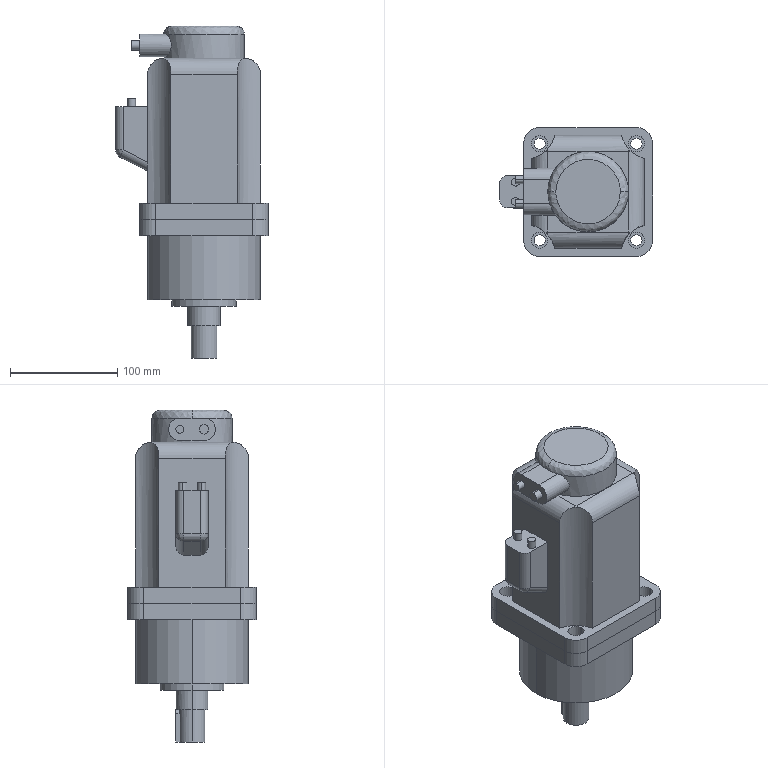Part | SolidWorks | features BaseBody 2, 3DProfileFeature 1, HoleWzd 1, ICE 1 | 2 solids | 132 faces | box 142.5 x 120 x 309 mm | volume 2592424 mm3 | cylinder 74 | plane 48 | spline 8 | cone 2 | commonest cylinder face diameters 7.5 x20 30 x14 15 x13 10.5 x8 60 x6 24 x3